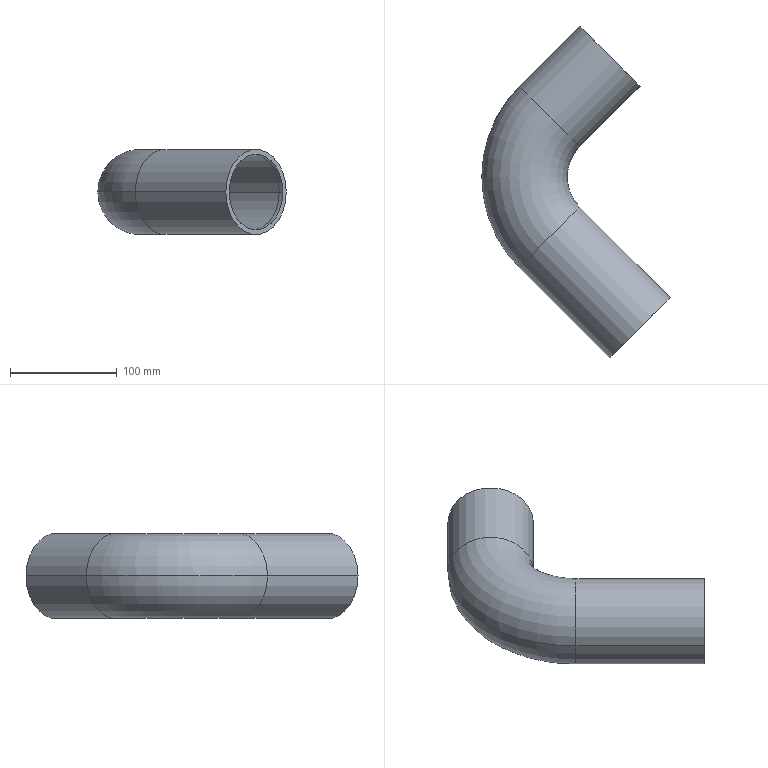Part | SolidWorks | 1 solid | 20 faces | box 176.563 x 311.125 x 80 mm | volume 356270 mm3 | cylinder 10 | torus 8 | plane 2 | commonest cylinder face diameters 70.758 x4 79.998 x4 70.756 x2
STEP:
#1=CARTESIAN_POINT('',(-62.081,461.178,-347.315));
#2=VERTEX_POINT('',#1);
#3=CARTESIAN_POINT('',(-62.082,461.177,-347.313));
#4=VERTEX_POINT('',#3);
#5=CARTESIAN_POINT('',(-37.064,486.195,-347.315));
#6=DIRECTION('',(-0.7071,0.7071,0.));
#7=DIRECTION('',(0.7071,0.7071,0.00003819));
#8=AXIS2_PLACEMENT_3D('',#5,#6,#7);
#9=CIRCLE('',#8,35.379);
#10=EDGE_CURVE('',#2,#4,#9,.T.);
#11=ORIENTED_EDGE('',*,*,#10,.F.);
#12=CARTESIAN_POINT('',(-62.081,624.345,-347.315));
#13=VERTEX_POINT('',#12);
#14=CARTESIAN_POINT('',(19.502,542.761,-347.315));
#15=DIRECTION('',(0.,0.,-1.));
#16=DIRECTION('',(-1.,0.,0.));
#17=AXIS2_PLACEMENT_3D('',#14,#15,#16);
#18=CIRCLE('',#17,115.376);
#19=EDGE_CURVE('',#2,#13,#18,.T.);
#20=ORIENTED_EDGE('',*,*,#19,.T.);
#21=CARTESIAN_POINT('',(-62.082,624.346,-347.313));
#22=VERTEX_POINT('',#21);
#23=CARTESIAN_POINT('',(-37.064,599.328,-347.315));
#24=DIRECTION('',(-0.7071,-0.7071,0.));
#25=DIRECTION('',(-0.7071,0.7071,0.00003818));
#26=AXIS2_PLACEMENT_3D('',#23,#24,#25);
#27=CIRCLE('',#26,35.379);
#28=EDGE_CURVE('',#22,#13,#27,.T.);
#29=ORIENTED_EDGE('',*,*,#28,.F.);
#30=CARTESIAN_POINT('',(19.502,542.761,-347.313));
#31=DIRECTION('',(0.,0.,1.));
#32=DIRECTION('',(-0.7071,0.7071,0.));
#33=AXIS2_PLACEMENT_3D('',#30,#31,#32);
#34=CIRCLE('',#33,115.376);
#35=EDGE_CURVE('',#22,#4,#34,.T.);
#36=ORIENTED_EDGE('',*,*,#35,.T.);
#37=EDGE_LOOP('',(#11,#20,#29,#36));
#38=FACE_OUTER_BOUND('',#37,.T.);
#39=CARTESIAN_POINT('',(19.502,542.761,-347.315));
#40=DIRECTION('',(0.,0.,-1.));
#41=DIRECTION('',(-0.7071,-0.7071,0.));
#42=AXIS2_PLACEMENT_3D('',#39,#40,#41);
#43=TOROIDAL_SURFACE('',#42,79.998,35.379);
#44=ADVANCED_FACE('',(#38),#43,.F.);
#45=ORIENTED_EDGE('',*,*,#19,.F.);
#46=CARTESIAN_POINT('',(-12.048,511.211,-347.315));
#47=VERTEX_POINT('',#46);
#48=CARTESIAN_POINT('',(-37.064,486.195,-347.315));
#49=DIRECTION('',(-0.7071,0.7071,0.));
#50=DIRECTION('',(0.7071,0.7071,0.00003819));
#51=AXIS2_PLACEMENT_3D('',#48,#49,#50);
#52=CIRCLE('',#51,35.379);
#53=EDGE_CURVE('',#47,#2,#52,.T.);
#54=ORIENTED_EDGE('',*,*,#53,.F.);
#55=CARTESIAN_POINT('',(-12.048,574.312,-347.315));
#56=VERTEX_POINT('',#55);
#57=CARTESIAN_POINT('',(19.502,542.761,-347.315));
#58=DIRECTION('',(0.,0.,-1.));
#59=DIRECTION('',(-1.,0.,0.));
#60=AXIS2_PLACEMENT_3D('',#57,#58,#59);
#61=CIRCLE('',#60,44.619);
#62=EDGE_CURVE('',#47,#56,#61,.T.);
#63=ORIENTED_EDGE('',*,*,#62,.T.);
#64=CARTESIAN_POINT('',(-37.064,599.328,-347.315));
#65=DIRECTION('',(-0.7071,-0.7071,0.));
#66=DIRECTION('',(-0.7071,0.7071,0.00003818));
#67=AXIS2_PLACEMENT_3D('',#64,#65,#66);
#68=CIRCLE('',#67,35.379);
#69=EDGE_CURVE('',#13,#56,#68,.T.);
#70=ORIENTED_EDGE('',*,*,#69,.F.);
#71=EDGE_LOOP('',(#45,#54,#63,#70));
#72=FACE_OUTER_BOUND('',#71,.T.);
#73=CARTESIAN_POINT('',(19.502,542.761,-347.315));
#74=DIRECTION('',(0.,0.,-1.));
#75=DIRECTION('',(-0.7071,-0.7071,0.));
#76=AXIS2_PLACEMENT_3D('',#73,#74,#75);
#77=TOROIDAL_SURFACE('',#76,79.998,35.379);
#78=ADVANCED_FACE('',(#72),#77,.F.);
#79=CARTESIAN_POINT('',(-62.081,624.345,-347.312));
#80=VERTEX_POINT('',#79);
#81=CARTESIAN_POINT('',(-37.064,599.328,-347.312));
#82=DIRECTION('',(-0.7071,-0.7071,0.));
#83=DIRECTION('',(0.7071,-0.7071,-0.00003819));
#84=AXIS2_PLACEMENT_3D('',#81,#82,#83);
#85=CIRCLE('',#84,35.379);
#86=EDGE_CURVE('',#80,#22,#85,.T.);
#87=ORIENTED_EDGE('',*,*,#86,.F.);
#88=CARTESIAN_POINT('',(-62.081,461.178,-347.312));
#89=VERTEX_POINT('',#88);
#90=CARTESIAN_POINT('',(19.502,542.761,-347.312));
#91=DIRECTION('',(0.,0.,1.));
#92=DIRECTION('',(1.,0.,0.));
#93=AXIS2_PLACEMENT_3D('',#90,#91,#92);
#94=CIRCLE('',#93,115.376);
#95=EDGE_CURVE('',#80,#89,#94,.T.);
#96=ORIENTED_EDGE('',*,*,#95,.T.);
#97=CARTESIAN_POINT('',(-37.064,486.195,-347.312));
#98=DIRECTION('',(-0.7071,0.7071,0.));
#99=DIRECTION('',(-0.7071,-0.7071,-0.00003818));
#100=AXIS2_PLACEMENT_3D('',#97,#98,#99);
#101=CIRCLE('',#100,35.379);
#102=EDGE_CURVE('',#4,#89,#101,.T.);
#103=ORIENTED_EDGE('',*,*,#102,.F.);
#104=ORIENTED_EDGE('',*,*,#35,.F.);
#105=EDGE_LOOP('',(#87,#96,#103,#104));
#106=FACE_OUTER_BOUND('',#105,.T.);
#107=CARTESIAN_POINT('',(19.502,542.761,-347.312));
#108=DIRECTION('',(0.,0.,1.));
#109=DIRECTION('',(-0.7071,-0.7071,0.));
#110=AXIS2_PLACEMENT_3D('',#107,#108,#109);
#111=TOROIDAL_SURFACE('',#110,79.998,35.379);
#112=ADVANCED_FACE('',(#106),#111,.F.);
#113=ORIENTED_EDGE('',*,*,#95,.F.);
#114=CARTESIAN_POINT('',(-12.048,574.312,-347.312));
#115=VERTEX_POINT('',#114);
#116=CARTESIAN_POINT('',(-37.064,599.328,-347.312));
#117=DIRECTION('',(-0.7071,-0.7071,0.));
#118=DIRECTION('',(0.7071,-0.7071,-0.00003819));
#119=AXIS2_PLACEMENT_3D('',#116,#117,#118);
#120=CIRCLE('',#119,35.379);
#121=EDGE_CURVE('',#115,#80,#120,.T.);
#122=ORIENTED_EDGE('',*,*,#121,.F.);
#123=CARTESIAN_POINT('',(-12.048,511.211,-347.312));
#124=VERTEX_POINT('',#123);
#125=CARTESIAN_POINT('',(19.502,542.761,-347.312));
#126=DIRECTION('',(0.,0.,1.));
#127=DIRECTION('',(1.,0.,0.));
#128=AXIS2_PLACEMENT_3D('',#125,#126,#127);
#129=CIRCLE('',#128,44.619);
#130=EDGE_CURVE('',#115,#124,#129,.T.);
#131=ORIENTED_EDGE('',*,*,#130,.T.);
#132=CARTESIAN_POINT('',(-37.064,486.195,-347.312));
#133=DIRECTION('',(-0.7071,0.7071,0.));
#134=DIRECTION('',(-0.7071,-0.7071,-0.00003818));
#135=AXIS2_PLACEMENT_3D('',#132,#133,#134);
#136=CIRCLE('',#135,35.379);
#137=EDGE_CURVE('',#89,#124,#136,.T.);
#138=ORIENTED_EDGE('',*,*,#137,.F.);
#139=EDGE_LOOP('',(#113,#122,#131,#138));
#140=FACE_OUTER_BOUND('',#139,.T.);
#141=CARTESIAN_POINT('',(19.502,542.761,-347.312));
#142=DIRECTION('',(0.,0.,1.));
#143=DIRECTION('',(-0.7071,-0.7071,0.));
#144=AXIS2_PLACEMENT_3D('',#141,#142,#143);
#145=TOROIDAL_SURFACE('',#144,79.998,35.379);
#146=ADVANCED_FACE('',(#140),#145,.F.);
#147=ORIENTED_EDGE('',*,*,#130,.F.);
#148=CARTESIAN_POINT('',(-12.049,574.313,-347.313));
#149=VERTEX_POINT('',#148);
#150=CARTESIAN_POINT('',(-37.064,599.328,-347.312));
#151=DIRECTION('',(-0.7071,-0.7071,0.));
#152=DIRECTION('',(0.7071,-0.7071,-0.00003819));
#153=AXIS2_PLACEMENT_3D('',#150,#151,#152);
#154=CIRCLE('',#153,35.379);
#155=EDGE_CURVE('',#149,#115,#154,.T.);
#156=ORIENTED_EDGE('',*,*,#155,.F.);
#157=CARTESIAN_POINT('',(-12.049,511.21,-347.313));
#158=VERTEX_POINT('',#157);
#159=CARTESIAN_POINT('',(19.502,542.761,-347.313));
#160=DIRECTION('',(0.,0.,1.));
#161=DIRECTION('',(-0.7071,0.7071,0.));
#162=AXIS2_PLACEMENT_3D('',#159,#160,#161);
#163=CIRCLE('',#162,44.619);
#164=EDGE_CURVE('',#149,#158,#163,.T.);
#165=ORIENTED_EDGE('',*,*,#164,.T.);
#166=CARTESIAN_POINT('',(-37.064,486.195,-347.312));
#167=DIRECTION('',(-0.7071,0.7071,0.));
#168=DIRECTION('',(-0.7071,-0.7071,-0.00003818));
#169=AXIS2_PLACEMENT_3D('',#166,#167,#168);
#170=CIRCLE('',#169,35.379);
#171=EDGE_CURVE('',#124,#158,#170,.T.);
#172=ORIENTED_EDGE('',*,*,#171,.F.);
#173=EDGE_LOOP('',(#147,#156,#165,#172));
#174=FACE_OUTER_BOUND('',#173,.T.);
#175=CARTESIAN_POINT('',(19.502,542.761,-347.312));
#176=DIRECTION('',(0.,0.,1.));
#177=DIRECTION('',(-0.7071,-0.7071,0.));
#178=AXIS2_PLACEMENT_3D('',#175,#176,#177);
#179=TOROIDAL_SURFACE('',#178,79.998,35.379);
#180=ADVANCED_FACE('',(#174),#179,.F.);
#181=ORIENTED_EDGE('',*,*,#62,.F.);
#182=CARTESIAN_POINT('',(-37.064,486.195,-347.315));
#183=DIRECTION('',(-0.7071,0.7071,0.));
#184=DIRECTION('',(0.7071,0.7071,0.00003819));
#185=AXIS2_PLACEMENT_3D('',#182,#183,#184);
#186=CIRCLE('',#185,35.379);
#187=EDGE_CURVE('',#158,#47,#186,.T.);
#188=ORIENTED_EDGE('',*,*,#187,.F.);
#189=ORIENTED_EDGE('',*,*,#164,.F.);
#190=CARTESIAN_POINT('',(-37.064,599.328,-347.315));
#191=DIRECTION('',(-0.7071,-0.7071,0.));
#192=DIRECTION('',(-0.7071,0.7071,0.00003818));
#193=AXIS2_PLACEMENT_3D('',#190,#191,#192);
#194=CIRCLE('',#193,35.379);
#195=EDGE_CURVE('',#56,#149,#194,.T.);
#196=ORIENTED_EDGE('',*,*,#195,.F.);
#197=EDGE_LOOP('',(#181,#188,#189,#196));
#198=FACE_OUTER_BOUND('',#197,.T.);
#199=CARTESIAN_POINT('',(19.502,542.761,-347.315));
#200=DIRECTION('',(0.,0.,-1.));
#201=DIRECTION('',(-0.7071,-0.7071,0.));
#202=AXIS2_PLACEMENT_3D('',#199,#200,#201);
#203=TOROIDAL_SURFACE('',#202,79.998,35.379);
#204=ADVANCED_FACE('',(#198),#203,.F.);
#205=ORIENTED_EDGE('',*,*,#28,.T.);
#206=ORIENTED_EDGE('',*,*,#69,.T.);
#207=ORIENTED_EDGE('',*,*,#195,.T.);
#208=CARTESIAN_POINT('',(44.519,630.882,-347.313));
#209=VERTEX_POINT('',#208);
#210=CARTESIAN_POINT('',(44.519,630.882,-347.313));
#211=DIRECTION('',(-0.7071,-0.7071,0.));
#212=VECTOR('',#211,1000.);
#213=LINE('',#210,#212);
#214=EDGE_CURVE('',#209,#149,#213,.T.);
#215=ORIENTED_EDGE('',*,*,#214,.F.);
#216=CARTESIAN_POINT('',(-5.514,680.915,-347.313));
#217=VERTEX_POINT('',#216);
#218=CARTESIAN_POINT('',(19.502,655.899,-347.313));
#219=DIRECTION('',(0.7071,0.7071,0.));
#220=DIRECTION('',(0.7071,-0.7071,0.000000001));
#221=AXIS2_PLACEMENT_3D('',#218,#219,#220);
#222=CIRCLE('',#221,35.379);
#223=EDGE_CURVE('',#209,#217,#222,.T.);
#224=ORIENTED_EDGE('',*,*,#223,.T.);
#225=CARTESIAN_POINT('',(-5.514,680.915,-347.313));
#226=DIRECTION('',(-0.7071,-0.7071,0.));
#227=VECTOR('',#226,1000.);
#228=LINE('',#225,#227);
#229=EDGE_CURVE('',#217,#22,#228,.T.);
#230=ORIENTED_EDGE('',*,*,#229,.T.);
#231=EDGE_LOOP('',(#205,#206,#207,#215,#224,#230));
#232=FACE_OUTER_BOUND('',#231,.T.);
#233=CARTESIAN_POINT('',(-8.782,627.614,-347.313));
#234=DIRECTION('',(0.7071,0.7071,0.));
#235=DIRECTION('',(0.7071,-0.7071,0.000000001));
#236=AXIS2_PLACEMENT_3D('',#233,#234,#235);
#237=CYLINDRICAL_SURFACE('',#236,35.379);
#238=ADVANCED_FACE('',(#232),#237,.F.);
#239=ORIENTED_EDGE('',*,*,#155,.T.);
#240=ORIENTED_EDGE('',*,*,#121,.T.);
#241=ORIENTED_EDGE('',*,*,#86,.T.);
#242=ORIENTED_EDGE('',*,*,#229,.F.);
#243=CARTESIAN_POINT('',(19.502,655.899,-347.313));
#244=DIRECTION('',(0.7071,0.7071,0.));
#245=DIRECTION('',(-0.7071,0.7071,-0.000000001));
#246=AXIS2_PLACEMENT_3D('',#243,#244,#245);
#247=CIRCLE('',#246,35.379);
#248=EDGE_CURVE('',#217,#209,#247,.T.);
#249=ORIENTED_EDGE('',*,*,#248,.T.);
#250=ORIENTED_EDGE('',*,*,#214,.T.);
#251=EDGE_LOOP('',(#239,#240,#241,#242,#249,#250));
#252=FACE_OUTER_BOUND('',#251,.T.);
#253=CARTESIAN_POINT('',(-8.782,627.614,-347.313));
#254=DIRECTION('',(0.7071,0.7071,0.));
#255=DIRECTION('',(-0.7071,0.7071,-0.000000001));
#256=AXIS2_PLACEMENT_3D('',#253,#254,#255);
#257=CYLINDRICAL_SURFACE('',#256,35.379);
#258=ADVANCED_FACE('',(#252),#257,.F.);
#259=ORIENTED_EDGE('',*,*,#223,.F.);
#260=ORIENTED_EDGE('',*,*,#248,.F.);
#261=EDGE_LOOP('',(#259,#260));
#262=FACE_BOUND('',#261,.T.);
#263=CARTESIAN_POINT('',(47.786,627.615,-347.313));
#264=VERTEX_POINT('',#263);
#265=CARTESIAN_POINT('',(-8.781,684.182,-347.313));
#266=VERTEX_POINT('',#265);
#267=CARTESIAN_POINT('',(19.502,655.899,-347.313));
#268=DIRECTION('',(-0.7071,-0.7071,0.));
#269=DIRECTION('',(0.7071,-0.7071,0.));
#270=AXIS2_PLACEMENT_3D('',#267,#268,#269);
#271=CIRCLE('',#270,39.999);
#272=EDGE_CURVE('',#264,#266,#271,.T.);
#273=ORIENTED_EDGE('',*,*,#272,.F.);
#274=CARTESIAN_POINT('',(19.502,655.899,-347.313));
#275=DIRECTION('',(-0.7071,-0.7071,0.));
#276=DIRECTION('',(-0.7071,0.7071,0.));
#277=AXIS2_PLACEMENT_3D('',#274,#275,#276);
#278=CIRCLE('',#277,39.999);
#279=EDGE_CURVE('',#266,#264,#278,.T.);
#280=ORIENTED_EDGE('',*,*,#279,.F.);
#281=EDGE_LOOP('',(#273,#280));
#282=FACE_OUTER_BOUND('',#281,.T.);
#283=CARTESIAN_POINT('',(-55.061,730.462,15.));
#284=DIRECTION('',(0.7071,0.7071,0.));
#285=DIRECTION('',(0.,0.,-1.));
#286=AXIS2_PLACEMENT_3D('',#283,#284,#285);
#287=PLANE('',#286);
#288=ADVANCED_FACE('',(#262,#282),#287,.T.);
#289=ORIENTED_EDGE('',*,*,#272,.T.);
#290=CARTESIAN_POINT('',(-65.348,627.612,-347.313));
#291=VERTEX_POINT('',#290);
#292=CARTESIAN_POINT('',(-8.781,684.182,-347.313));
#293=DIRECTION('',(-0.7071,-0.7071,0.));
#294=VECTOR('',#293,1000.);
#295=LINE('',#292,#294);
#296=EDGE_CURVE('',#266,#291,#295,.T.);
#297=ORIENTED_EDGE('',*,*,#296,.T.);
#298=CARTESIAN_POINT('',(-8.782,571.046,-347.313));
#299=VERTEX_POINT('',#298);
#300=CARTESIAN_POINT('',(-37.064,599.328,-347.311));
#301=DIRECTION('',(0.7071,0.7071,0.));
#302=DIRECTION('',(-0.7071,0.7071,-0.00006484));
#303=AXIS2_PLACEMENT_3D('',#300,#301,#302);
#304=CIRCLE('',#303,39.997);
#305=EDGE_CURVE('',#291,#299,#304,.T.);
#306=ORIENTED_EDGE('',*,*,#305,.T.);
#307=CARTESIAN_POINT('',(47.786,627.615,-347.313));
#308=DIRECTION('',(-0.7071,-0.7071,0.));
#309=VECTOR('',#308,1000.);
#310=LINE('',#307,#309);
#311=EDGE_CURVE('',#264,#299,#310,.T.);
#312=ORIENTED_EDGE('',*,*,#311,.F.);
#313=EDGE_LOOP('',(#289,#297,#306,#312));
#314=FACE_OUTER_BOUND('',#313,.T.);
#315=CARTESIAN_POINT('',(-8.782,627.614,-347.313));
#316=DIRECTION('',(0.7071,0.7071,0.));
#317=DIRECTION('',(-0.7071,0.7071,0.));
#318=AXIS2_PLACEMENT_3D('',#315,#316,#317);
#319=CYLINDRICAL_SURFACE('',#318,39.999);
#320=ADVANCED_FACE('',(#314),#319,.T.);
#321=ORIENTED_EDGE('',*,*,#279,.T.);
#322=ORIENTED_EDGE('',*,*,#311,.T.);
#323=CARTESIAN_POINT('',(-37.064,599.328,-347.316));
#324=DIRECTION('',(0.7071,0.7071,0.));
#325=DIRECTION('',(0.7071,-0.7071,0.00006485));
#326=AXIS2_PLACEMENT_3D('',#323,#324,#325);
#327=CIRCLE('',#326,39.997);
#328=EDGE_CURVE('',#299,#291,#327,.T.);
#329=ORIENTED_EDGE('',*,*,#328,.T.);
#330=ORIENTED_EDGE('',*,*,#296,.F.);
#331=EDGE_LOOP('',(#321,#322,#329,#330));
#332=FACE_OUTER_BOUND('',#331,.T.);
#333=CARTESIAN_POINT('',(-8.782,627.614,-347.313));
#334=DIRECTION('',(0.7071,0.7071,0.));
#335=DIRECTION('',(0.7071,-0.7071,0.));
#336=AXIS2_PLACEMENT_3D('',#333,#334,#335);
#337=CYLINDRICAL_SURFACE('',#336,39.999);
#338=ADVANCED_FACE('',(#332),#337,.T.);
#339=CARTESIAN_POINT('',(-65.348,457.911,-347.313));
#340=VERTEX_POINT('',#339);
#341=CARTESIAN_POINT('',(-8.782,514.477,-347.313));
#342=VERTEX_POINT('',#341);
#343=CARTESIAN_POINT('',(-37.064,486.195,-347.316));
#344=DIRECTION('',(0.7071,-0.7071,0.));
#345=DIRECTION('',(-0.7071,-0.7071,0.00006484));
#346=AXIS2_PLACEMENT_3D('',#343,#344,#345);
#347=CIRCLE('',#346,39.997);
#348=EDGE_CURVE('',#340,#342,#347,.T.);
#349=ORIENTED_EDGE('',*,*,#348,.F.);
#350=CARTESIAN_POINT('',(19.501,542.761,-347.313));
#351=DIRECTION('',(0.,0.,1.));
#352=DIRECTION('',(-0.7071,0.7071,0.));
#353=AXIS2_PLACEMENT_3D('',#350,#351,#352);
#354=CIRCLE('',#353,119.993);
#355=EDGE_CURVE('',#291,#340,#354,.T.);
#356=ORIENTED_EDGE('',*,*,#355,.F.);
#357=ORIENTED_EDGE('',*,*,#328,.F.);
#358=CARTESIAN_POINT('',(19.501,542.761,-347.313));
#359=DIRECTION('',(0.,0.,1.));
#360=DIRECTION('',(-0.7071,0.7071,0.));
#361=AXIS2_PLACEMENT_3D('',#358,#359,#360);
#362=CIRCLE('',#361,39.999);
#363=EDGE_CURVE('',#299,#342,#362,.T.);
#364=ORIENTED_EDGE('',*,*,#363,.T.);
#365=EDGE_LOOP('',(#349,#356,#357,#364));
#366=FACE_OUTER_BOUND('',#365,.T.);
#367=CARTESIAN_POINT('',(19.501,542.761,-347.316));
#368=DIRECTION('',(0.,0.,1.));
#369=DIRECTION('',(-0.7071,-0.7071,0.));
#370=AXIS2_PLACEMENT_3D('',#367,#368,#369);
#371=TOROIDAL_SURFACE('',#370,79.996,39.997);
#372=ADVANCED_FACE('',(#366),#371,.T.);
#373=CARTESIAN_POINT('',(-37.064,486.195,-347.311));
#374=DIRECTION('',(0.7071,-0.7071,0.));
#375=DIRECTION('',(0.7071,0.7071,-0.00006485));
#376=AXIS2_PLACEMENT_3D('',#373,#374,#375);
#377=CIRCLE('',#376,39.997);
#378=EDGE_CURVE('',#342,#340,#377,.T.);
#379=ORIENTED_EDGE('',*,*,#378,.F.);
#380=ORIENTED_EDGE('',*,*,#363,.F.);
#381=ORIENTED_EDGE('',*,*,#305,.F.);
#382=ORIENTED_EDGE('',*,*,#355,.T.);
#383=EDGE_LOOP('',(#379,#380,#381,#382));
#384=FACE_OUTER_BOUND('',#383,.T.);
#385=CARTESIAN_POINT('',(19.501,542.761,-347.311));
#386=DIRECTION('',(0.,0.,1.));
#387=DIRECTION('',(-0.7071,-0.7071,0.));
#388=AXIS2_PLACEMENT_3D('',#385,#386,#387);
#389=TOROIDAL_SURFACE('',#388,79.996,39.997);
#390=ADVANCED_FACE('',(#384),#389,.T.);
#391=CARTESIAN_POINT('',(19.503,373.057,-347.313));
#392=VERTEX_POINT('',#391);
#393=CARTESIAN_POINT('',(76.07,429.624,-347.313));
#394=VERTEX_POINT('',#393);
#395=CARTESIAN_POINT('',(47.787,401.34,-347.313));
#396=DIRECTION('',(-0.7071,0.7071,0.));
#397=DIRECTION('',(-0.7071,-0.7071,0.));
#398=AXIS2_PLACEMENT_3D('',#395,#396,#397);
#399=CIRCLE('',#398,39.999);
#400=EDGE_CURVE('',#392,#394,#399,.T.);
#401=ORIENTED_EDGE('',*,*,#400,.T.);
#402=CARTESIAN_POINT('',(-8.783,514.476,-347.313));
#403=DIRECTION('',(0.7071,-0.7071,0.));
#404=VECTOR('',#403,1000.);
#405=LINE('',#402,#404);
#406=EDGE_CURVE('',#342,#394,#405,.T.);
#407=ORIENTED_EDGE('',*,*,#406,.F.);
#408=ORIENTED_EDGE('',*,*,#378,.T.);
#409=CARTESIAN_POINT('',(-65.349,457.909,-347.313));
#410=DIRECTION('',(0.7071,-0.7071,0.));
#411=VECTOR('',#410,1000.);
#412=LINE('',#409,#411);
#413=EDGE_CURVE('',#340,#392,#412,.T.);
#414=ORIENTED_EDGE('',*,*,#413,.T.);
#415=EDGE_LOOP('',(#401,#407,#408,#414));
#416=FACE_OUTER_BOUND('',#415,.T.);
#417=CARTESIAN_POINT('',(5.36,443.767,-347.313));
#418=DIRECTION('',(-0.7071,0.7071,0.));
#419=DIRECTION('',(-0.7071,-0.7071,0.));
#420=AXIS2_PLACEMENT_3D('',#417,#418,#419);
#421=CYLINDRICAL_SURFACE('',#420,39.999);
#422=ADVANCED_FACE('',(#416),#421,.T.);
#423=CARTESIAN_POINT('',(47.787,401.34,-347.313));
#424=DIRECTION('',(-0.7071,0.7071,0.));
#425=DIRECTION('',(0.7071,0.7071,0.));
#426=AXIS2_PLACEMENT_3D('',#423,#424,#425);
#427=CIRCLE('',#426,39.999);
#428=EDGE_CURVE('',#394,#392,#427,.T.);
#429=ORIENTED_EDGE('',*,*,#428,.T.);
#430=ORIENTED_EDGE('',*,*,#413,.F.);
#431=ORIENTED_EDGE('',*,*,#348,.T.);
#432=ORIENTED_EDGE('',*,*,#406,.T.);
#433=EDGE_LOOP('',(#429,#430,#431,#432));
#434=FACE_OUTER_BOUND('',#433,.T.);
#435=CARTESIAN_POINT('',(5.36,443.767,-347.313));
#436=DIRECTION('',(-0.7071,0.7071,0.));
#437=DIRECTION('',(0.7071,0.7071,0.));
#438=AXIS2_PLACEMENT_3D('',#435,#436,#437);
#439=CYLINDRICAL_SURFACE('',#438,39.999);
#440=ADVANCED_FACE('',(#434),#439,.T.);
#441=CARTESIAN_POINT('',(22.771,376.324,-347.313));
#442=VERTEX_POINT('',#441);
#443=CARTESIAN_POINT('',(72.803,426.356,-347.313));
#444=VERTEX_POINT('',#443);
#445=CARTESIAN_POINT('',(47.787,401.34,-347.313));
#446=DIRECTION('',(0.7071,-0.7071,0.));
#447=DIRECTION('',(-0.7071,-0.7071,0.));
#448=AXIS2_PLACEMENT_3D('',#445,#446,#447);
#449=CIRCLE('',#448,35.378);
#450=EDGE_CURVE('',#442,#444,#449,.T.);
#451=ORIENTED_EDGE('',*,*,#450,.F.);
#452=CARTESIAN_POINT('',(47.787,401.34,-347.313));
#453=DIRECTION('',(0.7071,-0.7071,0.));
#454=DIRECTION('',(0.7071,0.7071,0.));
#455=AXIS2_PLACEMENT_3D('',#452,#453,#454);
#456=CIRCLE('',#455,35.378);
#457=EDGE_CURVE('',#444,#442,#456,.T.);
#458=ORIENTED_EDGE('',*,*,#457,.F.);
#459=EDGE_LOOP('',(#451,#458));
#460=FACE_BOUND('',#459,.T.);
#461=ORIENTED_EDGE('',*,*,#400,.F.);
#462=ORIENTED_EDGE('',*,*,#428,.F.);
#463=EDGE_LOOP('',(#461,#462));
#464=FACE_OUTER_BOUND('',#463,.T.);
#465=CARTESIAN_POINT('',(-26.777,326.777,15.));
#466=DIRECTION('',(-0.7071,0.7071,0.));
#467=DIRECTION('',(0.,0.,1.));
#468=AXIS2_PLACEMENT_3D('',#465,#466,#467);
#469=PLANE('',#468);
#470=ADVANCED_FACE('',(#460,#464),#469,.F.);
#471=CARTESIAN_POINT('',(69.536,429.623,-347.313));
#472=VERTEX_POINT('',#471);
#473=CARTESIAN_POINT('',(19.504,379.591,-347.313));
#474=VERTEX_POINT('',#473);
#475=CARTESIAN_POINT('',(44.52,404.607,-347.313));
#476=DIRECTION('',(0.7071,-0.7071,0.));
#477=DIRECTION('',(0.7071,0.7071,0.));
#478=AXIS2_PLACEMENT_3D('',#475,#476,#477);
#479=CIRCLE('',#478,35.378);
#480=EDGE_CURVE('',#472,#474,#479,.T.);
#481=ORIENTED_EDGE('',*,*,#480,.F.);
#482=CARTESIAN_POINT('',(69.536,429.623,-347.313));
#483=DIRECTION('',(0.7071,-0.7071,0.));
#484=VECTOR('',#483,1000.);
#485=LINE('',#482,#484);
#486=EDGE_CURVE('',#472,#444,#485,.T.);
#487=ORIENTED_EDGE('',*,*,#486,.T.);
#488=ORIENTED_EDGE('',*,*,#457,.T.);
#489=CARTESIAN_POINT('',(19.504,379.591,-347.313));
#490=DIRECTION('',(0.7071,-0.7071,0.));
#491=VECTOR('',#490,1000.);
#492=LINE('',#489,#491);
#493=EDGE_CURVE('',#474,#442,#492,.T.);
#494=ORIENTED_EDGE('',*,*,#493,.F.);
#495=EDGE_LOOP('',(#481,#487,#488,#494));
#496=FACE_OUTER_BOUND('',#495,.T.);
#497=CARTESIAN_POINT('',(54.858,394.269,-347.313));
#498=DIRECTION('',(-0.7071,0.7071,0.));
#499=DIRECTION('',(0.7071,0.7071,0.));
#500=AXIS2_PLACEMENT_3D('',#497,#498,#499);
#501=CYLINDRICAL_SURFACE('',#500,35.378);
#502=ADVANCED_FACE('',(#496),#501,.F.);
#503=CARTESIAN_POINT('',(44.52,404.607,-347.313));
#504=DIRECTION('',(0.7071,-0.7071,0.));
#505=DIRECTION('',(-0.7071,-0.7071,0.));
#506=AXIS2_PLACEMENT_3D('',#503,#504,#505);
#507=CIRCLE('',#506,35.378);
#508=EDGE_CURVE('',#474,#472,#507,.T.);
#509=ORIENTED_EDGE('',*,*,#508,.F.);
#510=ORIENTED_EDGE('',*,*,#493,.T.);
#511=ORIENTED_EDGE('',*,*,#450,.T.);
#512=ORIENTED_EDGE('',*,*,#486,.F.);
#513=EDGE_LOOP('',(#509,#510,#511,#512));
#514=FACE_OUTER_BOUND('',#513,.T.);
#515=CARTESIAN_POINT('',(54.858,394.269,-347.313));
#516=DIRECTION('',(-0.7071,0.7071,0.));
#517=DIRECTION('',(0.7071,0.7071,0.));
#518=AXIS2_PLACEMENT_3D('',#515,#516,#517);
#519=CYLINDRICAL_SURFACE('',#518,35.378);
#520=ADVANCED_FACE('',(#514),#519,.F.);
#521=ORIENTED_EDGE('',*,*,#187,.T.);
#522=ORIENTED_EDGE('',*,*,#53,.T.);
#523=ORIENTED_EDGE('',*,*,#10,.T.);
#524=CARTESIAN_POINT('',(-62.083,461.176,-347.313));
#525=DIRECTION('',(0.7071,-0.7071,0.));
#526=VECTOR('',#525,1000.);
#527=LINE('',#524,#526);
#528=EDGE_CURVE('',#4,#474,#527,.T.);
#529=ORIENTED_EDGE('',*,*,#528,.T.);
#530=ORIENTED_EDGE('',*,*,#508,.T.);
#531=CARTESIAN_POINT('',(-12.049,511.21,-347.313));
#532=DIRECTION('',(0.7071,-0.7071,0.));
#533=VECTOR('',#532,1000.);
#534=LINE('',#531,#533);
#535=EDGE_CURVE('',#158,#472,#534,.T.);
#536=ORIENTED_EDGE('',*,*,#535,.F.);
#537=EDGE_LOOP('',(#521,#522,#523,#529,#530,#536));
#538=FACE_OUTER_BOUND('',#537,.T.);
#539=CARTESIAN_POINT('',(3.727,445.4,-347.313));
#540=DIRECTION('',(-0.7071,0.7071,0.));
#541=DIRECTION('',(0.7071,0.7071,0.));
#542=AXIS2_PLACEMENT_3D('',#539,#540,#541);
#543=CYLINDRICAL_SURFACE('',#542,35.379);
#544=ADVANCED_FACE('',(#538),#543,.F.);
#545=ORIENTED_EDGE('',*,*,#102,.T.);
#546=ORIENTED_EDGE('',*,*,#137,.T.);
#547=ORIENTED_EDGE('',*,*,#171,.T.);
#548=ORIENTED_EDGE('',*,*,#535,.T.);
#549=ORIENTED_EDGE('',*,*,#480,.T.);
#550=ORIENTED_EDGE('',*,*,#528,.F.);
#551=EDGE_LOOP('',(#545,#546,#547,#548,#549,#550));
#552=FACE_OUTER_BOUND('',#551,.T.);
#553=CARTESIAN_POINT('',(3.727,445.4,-347.313));
#554=DIRECTION('',(-0.7071,0.7071,0.));
#555=DIRECTION('',(-0.7071,-0.7071,0.));
#556=AXIS2_PLACEMENT_3D('',#553,#554,#555);
#557=CYLINDRICAL_SURFACE('',#556,35.379);
#558=ADVANCED_FACE('',(#552),#557,.F.);
#559=CLOSED_SHELL('',(#44,#78,#112,#146,#180,#204,#238,#258,#288,#320,#338,#372,#390,#422,#440,#470,#502,#520,#544,#558));
#560=MANIFOLD_SOLID_BREP('',#559);
#561=CARTESIAN_POINT('',(0.,0.,0.));
#562=DIRECTION('',(0.,0.,1.));
#563=DIRECTION('',(1.,0.,0.));
#564=AXIS2_PLACEMENT_3D('',#561,#562,#563);
#565=(LENGTH_UNIT()NAMED_UNIT(*)SI_UNIT(.MILLI.,.METRE.));
#566=UNCERTAINTY_MEASURE_WITH_UNIT(LENGTH_MEASURE(0.00001),#565,'','');
#567=(NAMED_UNIT(*)PLANE_ANGLE_UNIT()SI_UNIT($,.RADIAN.));
#568=(NAMED_UNIT(*)SI_UNIT($,.STERADIAN.)SOLID_ANGLE_UNIT());
#569=(GEOMETRIC_REPRESENTATION_CONTEXT(3)GLOBAL_UNCERTAINTY_ASSIGNED_CONTEXT((#566))GLOBAL_UNIT_ASSIGNED_CONTEXT((#565,#567,#568))REPRESENTATION_CONTEXT('',''));
#570=ADVANCED_BREP_SHAPE_REPRESENTATION('',(#560,#564),#569);